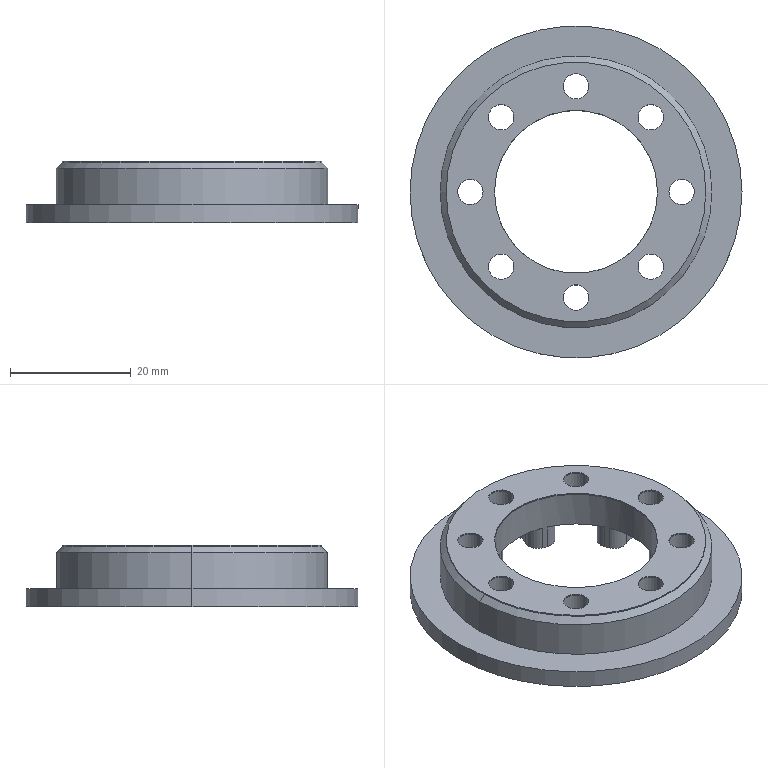Part | SolidWorks | features ICE 3, Chamfer 1, Fillet 1, Revolution 1 | 2 solids | 92 faces | box 55 x 55 x 10.2 mm | volume 10014 mm3 | cylinder 77 | plane 13 | cone 2 | commonest cylinder face diameters 4.2 x32 4 x20 8.5 x15 27 x4 43 x2 45 x2